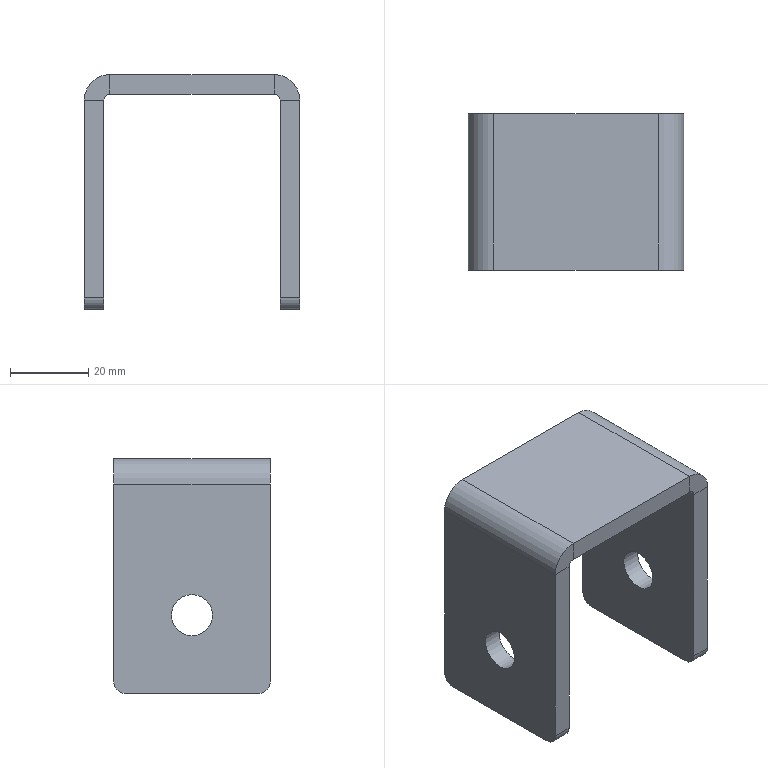Part | STEP file | 6150404 | 1 solid | 28 faces | box 55 x 40 x 60 mm | volume 31409 mm3 | plane 18 | cylinder 10 | commonest cylinder face diameters 6 x4 3 x2 10.5 x2 13 x2
STEP:
#1=CARTESIAN_POINT('',(22.5,3.,-30.));
#2=VERTEX_POINT('',#1);
#3=CARTESIAN_POINT('',(27.5,3.,-30.));
#4=VERTEX_POINT('',#3);
#5=CARTESIAN_POINT('',(-111.1,3.,-30.));
#6=DIRECTION('',(1.,0.,0.));
#7=VECTOR('',#6,1000.);
#8=LINE('',#5,#7);
#9=EDGE_CURVE('',#2,#4,#8,.T.);
#10=ORIENTED_EDGE('',*,*,#9,.T.);
#11=CARTESIAN_POINT('',(27.5,0.,-27.));
#12=VERTEX_POINT('',#11);
#13=CARTESIAN_POINT('',(27.5,3.,-27.));
#14=DIRECTION('',(1.,0.,0.));
#15=DIRECTION('',(0.,0.,1.));
#16=AXIS2_PLACEMENT_3D('',#13,#14,#15);
#17=CIRCLE('',#16,3.);
#18=EDGE_CURVE('',#12,#4,#17,.T.);
#19=ORIENTED_EDGE('',*,*,#18,.F.);
#20=CARTESIAN_POINT('',(22.5,0.,-27.));
#21=VERTEX_POINT('',#20);
#22=CARTESIAN_POINT('',(-111.1,0.,-27.));
#23=DIRECTION('',(1.,0.,0.));
#24=VECTOR('',#23,1000.);
#25=LINE('',#22,#24);
#26=EDGE_CURVE('',#21,#12,#25,.T.);
#27=ORIENTED_EDGE('',*,*,#26,.F.);
#28=CARTESIAN_POINT('',(22.5,3.,-27.));
#29=DIRECTION('',(-1.,0.,0.));
#30=DIRECTION('',(0.,0.,-1.));
#31=AXIS2_PLACEMENT_3D('',#28,#29,#30);
#32=CIRCLE('',#31,3.);
#33=EDGE_CURVE('',#2,#21,#32,.T.);
#34=ORIENTED_EDGE('',*,*,#33,.F.);
#35=EDGE_LOOP('',(#10,#19,#27,#34));
#36=FACE_OUTER_BOUND('',#35,.T.);
#37=CARTESIAN_POINT('',(-111.1,3.,-27.));
#38=DIRECTION('',(1.,0.,0.));
#39=DIRECTION('',(0.,0.,-1.));
#40=AXIS2_PLACEMENT_3D('',#37,#38,#39);
#41=CYLINDRICAL_SURFACE('',#40,3.);
#42=ADVANCED_FACE('',(#36),#41,.T.);
#43=CARTESIAN_POINT('',(22.5,37.,-30.));
#44=VERTEX_POINT('',#43);
#45=CARTESIAN_POINT('',(27.5,37.,-30.));
#46=VERTEX_POINT('',#45);
#47=CARTESIAN_POINT('',(-111.1,37.,-30.));
#48=DIRECTION('',(1.,0.,0.));
#49=VECTOR('',#48,1000.);
#50=LINE('',#47,#49);
#51=EDGE_CURVE('',#44,#46,#50,.T.);
#52=ORIENTED_EDGE('',*,*,#51,.T.);
#53=CARTESIAN_POINT('',(27.5,40.,-30.));
#54=DIRECTION('',(0.,-1.,0.));
#55=VECTOR('',#54,1000.);
#56=LINE('',#53,#55);
#57=EDGE_CURVE('',#46,#4,#56,.T.);
#58=ORIENTED_EDGE('',*,*,#57,.T.);
#59=ORIENTED_EDGE('',*,*,#9,.F.);
#60=CARTESIAN_POINT('',(22.5,40.,-30.));
#61=DIRECTION('',(0.,-1.,0.));
#62=VECTOR('',#61,1000.);
#63=LINE('',#60,#62);
#64=EDGE_CURVE('',#44,#2,#63,.T.);
#65=ORIENTED_EDGE('',*,*,#64,.F.);
#66=EDGE_LOOP('',(#52,#58,#59,#65));
#67=FACE_OUTER_BOUND('',#66,.T.);
#68=CARTESIAN_POINT('',(-111.1,40.,-30.));
#69=DIRECTION('',(0.,0.,1.));
#70=DIRECTION('',(1.,0.,0.));
#71=AXIS2_PLACEMENT_3D('',#68,#69,#70);
#72=PLANE('',#71);
#73=ADVANCED_FACE('',(#67),#72,.F.);
#74=CARTESIAN_POINT('',(22.5,20.,-15.25));
#75=VERTEX_POINT('',#74);
#76=CARTESIAN_POINT('',(22.5,20.,-10.));
#77=DIRECTION('',(1.,0.,0.));
#78=DIRECTION('',(0.,0.,-1.));
#79=AXIS2_PLACEMENT_3D('',#76,#77,#78);
#80=CIRCLE('',#79,5.25);
#81=EDGE_CURVE('',#75,#75,#80,.T.);
#82=ORIENTED_EDGE('',*,*,#81,.F.);
#83=EDGE_LOOP('',(#82));
#84=FACE_OUTER_BOUND('',#83,.T.);
#85=CARTESIAN_POINT('',(27.5,20.,-4.75));
#86=VERTEX_POINT('',#85);
#87=CARTESIAN_POINT('',(27.5,20.,-10.));
#88=DIRECTION('',(-1.,0.,0.));
#89=DIRECTION('',(0.,0.,1.));
#90=AXIS2_PLACEMENT_3D('',#87,#88,#89);
#91=CIRCLE('',#90,5.25);
#92=EDGE_CURVE('',#86,#86,#91,.T.);
#93=ORIENTED_EDGE('',*,*,#92,.F.);
#94=EDGE_LOOP('',(#93));
#95=FACE_OUTER_BOUND('',#94,.T.);
#96=CARTESIAN_POINT('',(36.5,20.,-10.));
#97=DIRECTION('',(-1.,0.,0.));
#98=DIRECTION('',(0.,0.,1.));
#99=AXIS2_PLACEMENT_3D('',#96,#97,#98);
#100=CYLINDRICAL_SURFACE('',#99,5.25);
#101=ADVANCED_FACE('',(#84,#95),#100,.F.);
#102=CARTESIAN_POINT('',(22.5,40.,-27.));
#103=VERTEX_POINT('',#102);
#104=CARTESIAN_POINT('',(27.5,40.,-27.));
#105=VERTEX_POINT('',#104);
#106=CARTESIAN_POINT('',(-111.1,40.,-27.));
#107=DIRECTION('',(1.,0.,0.));
#108=VECTOR('',#107,1000.);
#109=LINE('',#106,#108);
#110=EDGE_CURVE('',#103,#105,#109,.T.);
#111=ORIENTED_EDGE('',*,*,#110,.T.);
#112=CARTESIAN_POINT('',(27.5,37.,-27.));
#113=DIRECTION('',(1.,0.,0.));
#114=DIRECTION('',(0.,0.,1.));
#115=AXIS2_PLACEMENT_3D('',#112,#113,#114);
#116=CIRCLE('',#115,3.);
#117=EDGE_CURVE('',#46,#105,#116,.T.);
#118=ORIENTED_EDGE('',*,*,#117,.F.);
#119=ORIENTED_EDGE('',*,*,#51,.F.);
#120=CARTESIAN_POINT('',(22.5,37.,-27.));
#121=DIRECTION('',(-1.,0.,0.));
#122=DIRECTION('',(0.,0.,-1.));
#123=AXIS2_PLACEMENT_3D('',#120,#121,#122);
#124=CIRCLE('',#123,3.);
#125=EDGE_CURVE('',#103,#44,#124,.T.);
#126=ORIENTED_EDGE('',*,*,#125,.F.);
#127=EDGE_LOOP('',(#111,#118,#119,#126));
#128=FACE_OUTER_BOUND('',#127,.T.);
#129=CARTESIAN_POINT('',(-111.1,37.,-27.));
#130=DIRECTION('',(1.,0.,0.));
#131=DIRECTION('',(0.,0.,-1.));
#132=AXIS2_PLACEMENT_3D('',#129,#130,#131);
#133=CYLINDRICAL_SURFACE('',#132,3.);
#134=ADVANCED_FACE('',(#128),#133,.T.);
#135=CARTESIAN_POINT('',(27.5,40.,23.5));
#136=VERTEX_POINT('',#135);
#137=CARTESIAN_POINT('',(27.5,40.,-30.));
#138=DIRECTION('',(0.,0.,-1.));
#139=VECTOR('',#138,1000.);
#140=LINE('',#137,#139);
#141=EDGE_CURVE('',#136,#105,#140,.T.);
#142=ORIENTED_EDGE('',*,*,#141,.T.);
#143=ORIENTED_EDGE('',*,*,#110,.F.);
#144=CARTESIAN_POINT('',(22.5,40.,23.5));
#145=VERTEX_POINT('',#144);
#146=CARTESIAN_POINT('',(22.5,40.,-30.));
#147=DIRECTION('',(0.,0.,1.));
#148=VECTOR('',#147,1000.);
#149=LINE('',#146,#148);
#150=EDGE_CURVE('',#103,#145,#149,.T.);
#151=ORIENTED_EDGE('',*,*,#150,.T.);
#152=CARTESIAN_POINT('',(-111.1,40.,23.5));
#153=DIRECTION('',(1.,0.,0.));
#154=VECTOR('',#153,1000.);
#155=LINE('',#152,#154);
#156=EDGE_CURVE('',#145,#136,#155,.T.);
#157=ORIENTED_EDGE('',*,*,#156,.T.);
#158=EDGE_LOOP('',(#142,#143,#151,#157));
#159=FACE_OUTER_BOUND('',#158,.T.);
#160=CARTESIAN_POINT('',(-111.1,40.,-30.));
#161=DIRECTION('',(0.,1.,0.));
#162=DIRECTION('',(1.,0.,0.));
#163=AXIS2_PLACEMENT_3D('',#160,#161,#162);
#164=PLANE('',#163);
#165=ADVANCED_FACE('',(#159),#164,.T.);
#166=ORIENTED_EDGE('',*,*,#92,.T.);
#167=EDGE_LOOP('',(#166));
#168=FACE_BOUND('',#167,.T.);
#169=ORIENTED_EDGE('',*,*,#57,.F.);
#170=ORIENTED_EDGE('',*,*,#117,.T.);
#171=ORIENTED_EDGE('',*,*,#141,.F.);
#172=CARTESIAN_POINT('',(27.5,0.,23.5));
#173=VERTEX_POINT('',#172);
#174=CARTESIAN_POINT('',(27.5,40.,23.5));
#175=DIRECTION('',(0.,-1.,0.));
#176=VECTOR('',#175,1000.);
#177=LINE('',#174,#176);
#178=EDGE_CURVE('',#136,#173,#177,.T.);
#179=ORIENTED_EDGE('',*,*,#178,.T.);
#180=CARTESIAN_POINT('',(27.5,0.,-30.));
#181=DIRECTION('',(0.,0.,-1.));
#182=VECTOR('',#181,1000.);
#183=LINE('',#180,#182);
#184=EDGE_CURVE('',#173,#12,#183,.T.);
#185=ORIENTED_EDGE('',*,*,#184,.T.);
#186=ORIENTED_EDGE('',*,*,#18,.T.);
#187=EDGE_LOOP('',(#169,#170,#171,#179,#185,#186));
#188=FACE_OUTER_BOUND('',#187,.T.);
#189=CARTESIAN_POINT('',(27.5,40.,-30.));
#190=DIRECTION('',(-1.,0.,0.));
#191=DIRECTION('',(0.,0.,1.));
#192=AXIS2_PLACEMENT_3D('',#189,#190,#191);
#193=PLANE('',#192);
#194=ADVANCED_FACE('',(#168,#188),#193,.F.);
#195=ORIENTED_EDGE('',*,*,#26,.T.);
#196=ORIENTED_EDGE('',*,*,#184,.F.);
#197=CARTESIAN_POINT('',(22.5,0.,23.5));
#198=VERTEX_POINT('',#197);
#199=CARTESIAN_POINT('',(-111.1,0.,23.5));
#200=DIRECTION('',(1.,0.,0.));
#201=VECTOR('',#200,1000.);
#202=LINE('',#199,#201);
#203=EDGE_CURVE('',#198,#173,#202,.T.);
#204=ORIENTED_EDGE('',*,*,#203,.F.);
#205=CARTESIAN_POINT('',(22.5,0.,-30.));
#206=DIRECTION('',(0.,0.,1.));
#207=VECTOR('',#206,1000.);
#208=LINE('',#205,#207);
#209=EDGE_CURVE('',#21,#198,#208,.T.);
#210=ORIENTED_EDGE('',*,*,#209,.F.);
#211=EDGE_LOOP('',(#195,#196,#204,#210));
#212=FACE_OUTER_BOUND('',#211,.T.);
#213=CARTESIAN_POINT('',(-111.1,0.,-30.));
#214=DIRECTION('',(0.,1.,0.));
#215=DIRECTION('',(1.,0.,0.));
#216=AXIS2_PLACEMENT_3D('',#213,#214,#215);
#217=PLANE('',#216);
#218=ADVANCED_FACE('',(#212),#217,.F.);
#219=ORIENTED_EDGE('',*,*,#81,.T.);
#220=EDGE_LOOP('',(#219));
#221=FACE_BOUND('',#220,.T.);
#222=ORIENTED_EDGE('',*,*,#150,.F.);
#223=ORIENTED_EDGE('',*,*,#125,.T.);
#224=ORIENTED_EDGE('',*,*,#64,.T.);
#225=ORIENTED_EDGE('',*,*,#33,.T.);
#226=ORIENTED_EDGE('',*,*,#209,.T.);
#227=CARTESIAN_POINT('',(22.5,40.,23.5));
#228=DIRECTION('',(0.,-1.,0.));
#229=VECTOR('',#228,1000.);
#230=LINE('',#227,#229);
#231=EDGE_CURVE('',#145,#198,#230,.T.);
#232=ORIENTED_EDGE('',*,*,#231,.F.);
#233=EDGE_LOOP('',(#222,#223,#224,#225,#226,#232));
#234=FACE_OUTER_BOUND('',#233,.T.);
#235=CARTESIAN_POINT('',(22.5,40.,-30.));
#236=DIRECTION('',(1.,0.,0.));
#237=DIRECTION('',(0.,0.,-1.));
#238=AXIS2_PLACEMENT_3D('',#235,#236,#237);
#239=PLANE('',#238);
#240=ADVANCED_FACE('',(#221,#234),#239,.F.);
#241=CARTESIAN_POINT('',(-22.5,37.,-30.));
#242=VERTEX_POINT('',#241);
#243=CARTESIAN_POINT('',(-27.5,37.,-30.));
#244=VERTEX_POINT('',#243);
#245=CARTESIAN_POINT('',(111.1,37.,-30.));
#246=DIRECTION('',(-1.,0.,0.));
#247=VECTOR('',#246,1000.);
#248=LINE('',#245,#247);
#249=EDGE_CURVE('',#242,#244,#248,.T.);
#250=ORIENTED_EDGE('',*,*,#249,.T.);
#251=CARTESIAN_POINT('',(-27.5,40.,-27.));
#252=VERTEX_POINT('',#251);
#253=CARTESIAN_POINT('',(-27.5,37.,-27.));
#254=DIRECTION('',(-1.,0.,0.));
#255=DIRECTION('',(0.,0.,-1.));
#256=AXIS2_PLACEMENT_3D('',#253,#254,#255);
#257=CIRCLE('',#256,3.);
#258=EDGE_CURVE('',#252,#244,#257,.T.);
#259=ORIENTED_EDGE('',*,*,#258,.F.);
#260=CARTESIAN_POINT('',(-22.5,40.,-27.));
#261=VERTEX_POINT('',#260);
#262=CARTESIAN_POINT('',(111.1,40.,-27.));
#263=DIRECTION('',(-1.,0.,0.));
#264=VECTOR('',#263,1000.);
#265=LINE('',#262,#264);
#266=EDGE_CURVE('',#261,#252,#265,.T.);
#267=ORIENTED_EDGE('',*,*,#266,.F.);
#268=CARTESIAN_POINT('',(-22.5,37.,-27.));
#269=DIRECTION('',(1.,0.,0.));
#270=DIRECTION('',(0.,0.,1.));
#271=AXIS2_PLACEMENT_3D('',#268,#269,#270);
#272=CIRCLE('',#271,3.);
#273=EDGE_CURVE('',#242,#261,#272,.T.);
#274=ORIENTED_EDGE('',*,*,#273,.F.);
#275=EDGE_LOOP('',(#250,#259,#267,#274));
#276=FACE_OUTER_BOUND('',#275,.T.);
#277=CARTESIAN_POINT('',(111.1,37.,-27.));
#278=DIRECTION('',(-1.,0.,0.));
#279=DIRECTION('',(0.,0.,1.));
#280=AXIS2_PLACEMENT_3D('',#277,#278,#279);
#281=CYLINDRICAL_SURFACE('',#280,3.);
#282=ADVANCED_FACE('',(#276),#281,.T.);
#283=CARTESIAN_POINT('',(-27.5,3.,-30.));
#284=VERTEX_POINT('',#283);
#285=CARTESIAN_POINT('',(-27.5,40.,-30.));
#286=DIRECTION('',(0.,-1.,0.));
#287=VECTOR('',#286,1000.);
#288=LINE('',#285,#287);
#289=EDGE_CURVE('',#244,#284,#288,.T.);
#290=ORIENTED_EDGE('',*,*,#289,.F.);
#291=ORIENTED_EDGE('',*,*,#249,.F.);
#292=CARTESIAN_POINT('',(-22.5,3.,-30.));
#293=VERTEX_POINT('',#292);
#294=CARTESIAN_POINT('',(-22.5,40.,-30.));
#295=DIRECTION('',(0.,-1.,0.));
#296=VECTOR('',#295,1000.);
#297=LINE('',#294,#296);
#298=EDGE_CURVE('',#242,#293,#297,.T.);
#299=ORIENTED_EDGE('',*,*,#298,.T.);
#300=CARTESIAN_POINT('',(111.1,3.,-30.));
#301=DIRECTION('',(-1.,0.,0.));
#302=VECTOR('',#301,1000.);
#303=LINE('',#300,#302);
#304=EDGE_CURVE('',#293,#284,#303,.T.);
#305=ORIENTED_EDGE('',*,*,#304,.T.);
#306=EDGE_LOOP('',(#290,#291,#299,#305));
#307=FACE_OUTER_BOUND('',#306,.T.);
#308=CARTESIAN_POINT('',(111.1,40.,-30.));
#309=DIRECTION('',(0.,0.,-1.));
#310=DIRECTION('',(-1.,0.,0.));
#311=AXIS2_PLACEMENT_3D('',#308,#309,#310);
#312=PLANE('',#311);
#313=ADVANCED_FACE('',(#307),#312,.T.);
#314=CARTESIAN_POINT('',(-27.5,20.,-4.75));
#315=VERTEX_POINT('',#314);
#316=CARTESIAN_POINT('',(-27.5,20.,-10.));
#317=DIRECTION('',(-1.,0.,0.));
#318=DIRECTION('',(0.,0.,1.));
#319=AXIS2_PLACEMENT_3D('',#316,#317,#318);
#320=CIRCLE('',#319,5.25);
#321=EDGE_CURVE('',#315,#315,#320,.T.);
#322=ORIENTED_EDGE('',*,*,#321,.T.);
#323=EDGE_LOOP('',(#322));
#324=FACE_OUTER_BOUND('',#323,.T.);
#325=CARTESIAN_POINT('',(-22.5,20.,-4.75));
#326=VERTEX_POINT('',#325);
#327=CARTESIAN_POINT('',(-22.5,20.,-10.));
#328=DIRECTION('',(-1.,0.,0.));
#329=DIRECTION('',(0.,0.,1.));
#330=AXIS2_PLACEMENT_3D('',#327,#328,#329);
#331=CIRCLE('',#330,5.25);
#332=EDGE_CURVE('',#326,#326,#331,.T.);
#333=ORIENTED_EDGE('',*,*,#332,.F.);
#334=EDGE_LOOP('',(#333));
#335=FACE_OUTER_BOUND('',#334,.T.);
#336=CARTESIAN_POINT('',(36.5,20.,-10.));
#337=DIRECTION('',(-1.,0.,0.));
#338=DIRECTION('',(0.,0.,1.));
#339=AXIS2_PLACEMENT_3D('',#336,#337,#338);
#340=CYLINDRICAL_SURFACE('',#339,5.25);
#341=ADVANCED_FACE('',(#324,#335),#340,.F.);
#342=CARTESIAN_POINT('',(-22.5,0.,-27.));
#343=VERTEX_POINT('',#342);
#344=CARTESIAN_POINT('',(-27.5,0.,-27.));
#345=VERTEX_POINT('',#344);
#346=CARTESIAN_POINT('',(111.1,0.,-27.));
#347=DIRECTION('',(-1.,0.,0.));
#348=VECTOR('',#347,1000.);
#349=LINE('',#346,#348);
#350=EDGE_CURVE('',#343,#345,#349,.T.);
#351=ORIENTED_EDGE('',*,*,#350,.T.);
#352=CARTESIAN_POINT('',(-27.5,3.,-27.));
#353=DIRECTION('',(-1.,0.,0.));
#354=DIRECTION('',(0.,0.,-1.));
#355=AXIS2_PLACEMENT_3D('',#352,#353,#354);
#356=CIRCLE('',#355,3.);
#357=EDGE_CURVE('',#284,#345,#356,.T.);
#358=ORIENTED_EDGE('',*,*,#357,.F.);
#359=ORIENTED_EDGE('',*,*,#304,.F.);
#360=CARTESIAN_POINT('',(-22.5,3.,-27.));
#361=DIRECTION('',(1.,0.,0.));
#362=DIRECTION('',(0.,0.,1.));
#363=AXIS2_PLACEMENT_3D('',#360,#361,#362);
#364=CIRCLE('',#363,3.);
#365=EDGE_CURVE('',#343,#293,#364,.T.);
#366=ORIENTED_EDGE('',*,*,#365,.F.);
#367=EDGE_LOOP('',(#351,#358,#359,#366));
#368=FACE_OUTER_BOUND('',#367,.T.);
#369=CARTESIAN_POINT('',(111.1,3.,-27.));
#370=DIRECTION('',(-1.,0.,0.));
#371=DIRECTION('',(0.,0.,1.));
#372=AXIS2_PLACEMENT_3D('',#369,#370,#371);
#373=CYLINDRICAL_SURFACE('',#372,3.);
#374=ADVANCED_FACE('',(#368),#373,.T.);
#375=CARTESIAN_POINT('',(-22.5,0.,23.5));
#376=VERTEX_POINT('',#375);
#377=CARTESIAN_POINT('',(-27.5,0.,23.5));
#378=VERTEX_POINT('',#377);
#379=CARTESIAN_POINT('',(111.1,0.,23.5));
#380=DIRECTION('',(-1.,0.,0.));
#381=VECTOR('',#380,1000.);
#382=LINE('',#379,#381);
#383=EDGE_CURVE('',#376,#378,#382,.T.);
#384=ORIENTED_EDGE('',*,*,#383,.T.);
#385=CARTESIAN_POINT('',(-27.5,0.,-30.));
#386=DIRECTION('',(0.,0.,1.));
#387=VECTOR('',#386,1000.);
#388=LINE('',#385,#387);
#389=EDGE_CURVE('',#345,#378,#388,.T.);
#390=ORIENTED_EDGE('',*,*,#389,.F.);
#391=ORIENTED_EDGE('',*,*,#350,.F.);
#392=CARTESIAN_POINT('',(-22.5,0.,-30.));
#393=DIRECTION('',(0.,0.,-1.));
#394=VECTOR('',#393,1000.);
#395=LINE('',#392,#394);
#396=EDGE_CURVE('',#376,#343,#395,.T.);
#397=ORIENTED_EDGE('',*,*,#396,.F.);
#398=EDGE_LOOP('',(#384,#390,#391,#397));
#399=FACE_OUTER_BOUND('',#398,.T.);
#400=CARTESIAN_POINT('',(111.1,0.,-30.));
#401=DIRECTION('',(0.,1.,0.));
#402=DIRECTION('',(-1.,0.,0.));
#403=AXIS2_PLACEMENT_3D('',#400,#401,#402);
#404=PLANE('',#403);
#405=ADVANCED_FACE('',(#399),#404,.F.);
#406=ORIENTED_EDGE('',*,*,#321,.F.);
#407=EDGE_LOOP('',(#406));
#408=FACE_BOUND('',#407,.T.);
#409=ORIENTED_EDGE('',*,*,#289,.T.);
#410=ORIENTED_EDGE('',*,*,#357,.T.);
#411=ORIENTED_EDGE('',*,*,#389,.T.);
#412=CARTESIAN_POINT('',(-27.5,40.,23.5));
#413=VERTEX_POINT('',#412);
#414=CARTESIAN_POINT('',(-27.5,40.,23.5));
#415=DIRECTION('',(0.,-1.,0.));
#416=VECTOR('',#415,1000.);
#417=LINE('',#414,#416);
#418=EDGE_CURVE('',#413,#378,#417,.T.);
#419=ORIENTED_EDGE('',*,*,#418,.F.);
#420=CARTESIAN_POINT('',(-27.5,40.,-30.));
#421=DIRECTION('',(0.,0.,1.));
#422=VECTOR('',#421,1000.);
#423=LINE('',#420,#422);
#424=EDGE_CURVE('',#252,#413,#423,.T.);
#425=ORIENTED_EDGE('',*,*,#424,.F.);
#426=ORIENTED_EDGE('',*,*,#258,.T.);
#427=EDGE_LOOP('',(#409,#410,#411,#419,#425,#426));
#428=FACE_OUTER_BOUND('',#427,.T.);
#429=CARTESIAN_POINT('',(-27.5,40.,-30.));
#430=DIRECTION('',(1.,0.,0.));
#431=DIRECTION('',(0.,0.,-1.));
#432=AXIS2_PLACEMENT_3D('',#429,#430,#431);
#433=PLANE('',#432);
#434=ADVANCED_FACE('',(#408,#428),#433,.F.);
#435=ORIENTED_EDGE('',*,*,#424,.T.);
#436=CARTESIAN_POINT('',(-22.5,40.,23.5));
#437=VERTEX_POINT('',#436);
#438=CARTESIAN_POINT('',(111.1,40.,23.5));
#439=DIRECTION('',(-1.,0.,0.));
#440=VECTOR('',#439,1000.);
#441=LINE('',#438,#440);
#442=EDGE_CURVE('',#437,#413,#441,.T.);
#443=ORIENTED_EDGE('',*,*,#442,.F.);
#444=CARTESIAN_POINT('',(-22.5,40.,-30.));
#445=DIRECTION('',(0.,0.,-1.));
#446=VECTOR('',#445,1000.);
#447=LINE('',#444,#446);
#448=EDGE_CURVE('',#437,#261,#447,.T.);
#449=ORIENTED_EDGE('',*,*,#448,.T.);
#450=ORIENTED_EDGE('',*,*,#266,.T.);
#451=EDGE_LOOP('',(#435,#443,#449,#450));
#452=FACE_OUTER_BOUND('',#451,.T.);
#453=CARTESIAN_POINT('',(111.1,40.,-30.));
#454=DIRECTION('',(0.,1.,0.));
#455=DIRECTION('',(-1.,0.,0.));
#456=AXIS2_PLACEMENT_3D('',#453,#454,#455);
#457=PLANE('',#456);
#458=ADVANCED_FACE('',(#452),#457,.T.);
#459=ORIENTED_EDGE('',*,*,#332,.T.);
#460=EDGE_LOOP('',(#459));
#461=FACE_BOUND('',#460,.T.);
#462=ORIENTED_EDGE('',*,*,#396,.T.);
#463=ORIENTED_EDGE('',*,*,#365,.T.);
#464=ORIENTED_EDGE('',*,*,#298,.F.);
#465=ORIENTED_EDGE('',*,*,#273,.T.);
#466=ORIENTED_EDGE('',*,*,#448,.F.);
#467=CARTESIAN_POINT('',(-22.5,40.,23.5));
#468=DIRECTION('',(0.,-1.,0.));
#469=VECTOR('',#468,1000.);
#470=LINE('',#467,#469);
#471=EDGE_CURVE('',#437,#376,#470,.T.);
#472=ORIENTED_EDGE('',*,*,#471,.T.);
#473=EDGE_LOOP('',(#462,#463,#464,#465,#466,#472));
#474=FACE_OUTER_BOUND('',#473,.T.);
#475=CARTESIAN_POINT('',(-22.5,40.,-30.));
#476=DIRECTION('',(-1.,0.,0.));
#477=DIRECTION('',(0.,0.,1.));
#478=AXIS2_PLACEMENT_3D('',#475,#476,#477);
#479=PLANE('',#478);
#480=ADVANCED_FACE('',(#461,#474),#479,.F.);
#481=CARTESIAN_POINT('',(-21.,0.,30.));
#482=VERTEX_POINT('',#481);
#483=CARTESIAN_POINT('',(21.,0.,30.));
#484=VERTEX_POINT('',#483);
#485=CARTESIAN_POINT('',(-21.,0.,30.));
#486=DIRECTION('',(1.,0.,0.));
#487=VECTOR('',#486,1000.);
#488=LINE('',#485,#487);
#489=EDGE_CURVE('',#482,#484,#488,.T.);
#490=ORIENTED_EDGE('',*,*,#489,.T.);
#491=CARTESIAN_POINT('',(21.,40.,30.));
#492=VERTEX_POINT('',#491);
#493=CARTESIAN_POINT('',(21.,40.,30.));
#494=DIRECTION('',(0.,-1.,0.));
#495=VECTOR('',#494,1000.);
#496=LINE('',#493,#495);
#497=EDGE_CURVE('',#492,#484,#496,.T.);
#498=ORIENTED_EDGE('',*,*,#497,.F.);
#499=CARTESIAN_POINT('',(-21.,40.,30.));
#500=VERTEX_POINT('',#499);
#501=CARTESIAN_POINT('',(-21.,40.,30.));
#502=DIRECTION('',(1.,0.,0.));
#503=VECTOR('',#502,1000.);
#504=LINE('',#501,#503);
#505=EDGE_CURVE('',#500,#492,#504,.T.);
#506=ORIENTED_EDGE('',*,*,#505,.F.);
#507=CARTESIAN_POINT('',(-21.,40.,30.));
#508=DIRECTION('',(0.,-1.,0.));
#509=VECTOR('',#508,1000.);
#510=LINE('',#507,#509);
#511=EDGE_CURVE('',#500,#482,#510,.T.);
#512=ORIENTED_EDGE('',*,*,#511,.T.);
#513=EDGE_LOOP('',(#490,#498,#506,#512));
#514=FACE_OUTER_BOUND('',#513,.T.);
#515=CARTESIAN_POINT('',(-21.,40.,30.));
#516=DIRECTION('',(0.,0.,-1.));
#517=DIRECTION('',(-1.,0.,0.));
#518=AXIS2_PLACEMENT_3D('',#515,#516,#517);
#519=PLANE('',#518);
#520=ADVANCED_FACE('',(#514),#519,.F.);
#521=CARTESIAN_POINT('',(21.,0.,25.));
#522=VERTEX_POINT('',#521);
#523=CARTESIAN_POINT('',(-21.,0.,25.));
#524=VERTEX_POINT('',#523);
#525=CARTESIAN_POINT('',(-21.,0.,25.));
#526=DIRECTION('',(-1.,0.,0.));
#527=VECTOR('',#526,1000.);
#528=LINE('',#525,#527);
#529=EDGE_CURVE('',#522,#524,#528,.T.);
#530=ORIENTED_EDGE('',*,*,#529,.T.);
#531=CARTESIAN_POINT('',(-21.,40.,25.));
#532=VERTEX_POINT('',#531);
#533=CARTESIAN_POINT('',(-21.,40.,25.));
#534=DIRECTION('',(0.,-1.,0.));
#535=VECTOR('',#534,1000.);
#536=LINE('',#533,#535);
#537=EDGE_CURVE('',#532,#524,#536,.T.);
#538=ORIENTED_EDGE('',*,*,#537,.F.);
#539=CARTESIAN_POINT('',(21.,40.,25.));
#540=VERTEX_POINT('',#539);
#541=CARTESIAN_POINT('',(-21.,40.,25.));
#542=DIRECTION('',(-1.,0.,0.));
#543=VECTOR('',#542,1000.);
#544=LINE('',#541,#543);
#545=EDGE_CURVE('',#540,#532,#544,.T.);
#546=ORIENTED_EDGE('',*,*,#545,.F.);
#547=CARTESIAN_POINT('',(21.,40.,25.));
#548=DIRECTION('',(0.,-1.,0.));
#549=VECTOR('',#548,1000.);
#550=LINE('',#547,#549);
#551=EDGE_CURVE('',#540,#522,#550,.T.);
#552=ORIENTED_EDGE('',*,*,#551,.T.);
#553=EDGE_LOOP('',(#530,#538,#546,#552));
#554=FACE_OUTER_BOUND('',#553,.T.);
#555=CARTESIAN_POINT('',(-21.,40.,25.));
#556=DIRECTION('',(0.,0.,1.));
#557=DIRECTION('',(1.,0.,0.));
#558=AXIS2_PLACEMENT_3D('',#555,#556,#557);
#559=PLANE('',#558);
#560=ADVANCED_FACE('',(#554),#559,.F.);
#561=CARTESIAN_POINT('',(21.,0.,-91.));
#562=DIRECTION('',(0.,0.,1.));
#563=VECTOR('',#562,1000.);
#564=LINE('',#561,#563);
#565=EDGE_CURVE('',#522,#484,#564,.T.);
#566=ORIENTED_EDGE('',*,*,#565,.T.);
#567=ORIENTED_EDGE('',*,*,#489,.F.);
#568=CARTESIAN_POINT('',(-21.,0.,-91.));
#569=DIRECTION('',(0.,0.,1.));
#570=VECTOR('',#569,1000.);
#571=LINE('',#568,#570);
#572=EDGE_CURVE('',#524,#482,#571,.T.);
#573=ORIENTED_EDGE('',*,*,#572,.F.);
#574=ORIENTED_EDGE('',*,*,#529,.F.);
#575=EDGE_LOOP('',(#566,#567,#573,#574));
#576=FACE_OUTER_BOUND('',#575,.T.);
#577=CARTESIAN_POINT('',(-21.,0.,-91.));
#578=DIRECTION('',(0.,1.,0.));
#579=DIRECTION('',(0.,0.,1.));
#580=AXIS2_PLACEMENT_3D('',#577,#578,#579);
#581=PLANE('',#580);
#582=ADVANCED_FACE('',(#576),#581,.F.);
#583=ORIENTED_EDGE('',*,*,#505,.T.);
#584=CARTESIAN_POINT('',(21.,40.,-91.));
#585=DIRECTION('',(0.,0.,1.));
#586=VECTOR('',#585,1000.);
#587=LINE('',#584,#586);
#588=EDGE_CURVE('',#540,#492,#587,.T.);
#589=ORIENTED_EDGE('',*,*,#588,.F.);
#590=ORIENTED_EDGE('',*,*,#545,.T.);
#591=CARTESIAN_POINT('',(-21.,40.,-91.));
#592=DIRECTION('',(0.,0.,1.));
#593=VECTOR('',#592,1000.);
#594=LINE('',#591,#593);
#595=EDGE_CURVE('',#532,#500,#594,.T.);
#596=ORIENTED_EDGE('',*,*,#595,.T.);
#597=EDGE_LOOP('',(#583,#589,#590,#596));
#598=FACE_OUTER_BOUND('',#597,.T.);
#599=CARTESIAN_POINT('',(-21.,40.,-91.));
#600=DIRECTION('',(0.,1.,0.));
#601=DIRECTION('',(0.,0.,1.));
#602=AXIS2_PLACEMENT_3D('',#599,#600,#601);
#603=PLANE('',#602);
#604=ADVANCED_FACE('',(#598),#603,.T.);
#605=ORIENTED_EDGE('',*,*,#383,.F.);
#606=CARTESIAN_POINT('',(-21.,0.,23.5));
#607=DIRECTION('',(0.,1.,0.));
#608=DIRECTION('',(0.,0.,1.));
#609=AXIS2_PLACEMENT_3D('',#606,#607,#608);
#610=CIRCLE('',#609,1.5);
#611=EDGE_CURVE('',#376,#524,#610,.T.);
#612=ORIENTED_EDGE('',*,*,#611,.T.);
#613=ORIENTED_EDGE('',*,*,#572,.T.);
#614=CARTESIAN_POINT('',(-21.,0.,23.5));
#615=DIRECTION('',(0.,1.,0.));
#616=DIRECTION('',(0.,0.,1.));
#617=AXIS2_PLACEMENT_3D('',#614,#615,#616);
#618=CIRCLE('',#617,6.5);
#619=EDGE_CURVE('',#378,#482,#618,.T.);
#620=ORIENTED_EDGE('',*,*,#619,.F.);
#621=EDGE_LOOP('',(#605,#612,#613,#620));
#622=FACE_OUTER_BOUND('',#621,.T.);
#623=CARTESIAN_POINT('',(-21.,0.,23.5));
#624=DIRECTION('',(0.,-1.,0.));
#625=DIRECTION('',(0.,0.,-1.));
#626=AXIS2_PLACEMENT_3D('',#623,#624,#625);
#627=PLANE('',#626);
#628=ADVANCED_FACE('',(#622),#627,.T.);
#629=CARTESIAN_POINT('',(-21.,40.,23.5));
#630=DIRECTION('',(0.,-1.,0.));
#631=DIRECTION('',(0.,0.,1.));
#632=AXIS2_PLACEMENT_3D('',#629,#630,#631);
#633=CIRCLE('',#632,1.5);
#634=EDGE_CURVE('',#532,#437,#633,.T.);
#635=ORIENTED_EDGE('',*,*,#634,.T.);
#636=ORIENTED_EDGE('',*,*,#442,.T.);
#637=CARTESIAN_POINT('',(-21.,40.,23.5));
#638=DIRECTION('',(0.,-1.,0.));
#639=DIRECTION('',(0.,0.,1.));
#640=AXIS2_PLACEMENT_3D('',#637,#638,#639);
#641=CIRCLE('',#640,6.5);
#642=EDGE_CURVE('',#500,#413,#641,.T.);
#643=ORIENTED_EDGE('',*,*,#642,.F.);
#644=ORIENTED_EDGE('',*,*,#595,.F.);
#645=EDGE_LOOP('',(#635,#636,#643,#644));
#646=FACE_OUTER_BOUND('',#645,.T.);
#647=CARTESIAN_POINT('',(-21.,40.,23.5));
#648=DIRECTION('',(0.,1.,0.));
#649=DIRECTION('',(0.,0.,1.));
#650=AXIS2_PLACEMENT_3D('',#647,#648,#649);
#651=PLANE('',#650);
#652=ADVANCED_FACE('',(#646),#651,.T.);
#653=ORIENTED_EDGE('',*,*,#511,.F.);
#654=ORIENTED_EDGE('',*,*,#642,.T.);
#655=ORIENTED_EDGE('',*,*,#418,.T.);
#656=ORIENTED_EDGE('',*,*,#619,.T.);
#657=EDGE_LOOP('',(#653,#654,#655,#656));
#658=FACE_OUTER_BOUND('',#657,.T.);
#659=CARTESIAN_POINT('',(-21.,-166.519,23.5));
#660=DIRECTION('',(0.,1.,0.));
#661=DIRECTION('',(0.,0.,1.));
#662=AXIS2_PLACEMENT_3D('',#659,#660,#661);
#663=CYLINDRICAL_SURFACE('',#662,6.5);
#664=ADVANCED_FACE('',(#658),#663,.T.);
#665=ORIENTED_EDGE('',*,*,#537,.T.);
#666=ORIENTED_EDGE('',*,*,#611,.F.);
#667=ORIENTED_EDGE('',*,*,#471,.F.);
#668=ORIENTED_EDGE('',*,*,#634,.F.);
#669=EDGE_LOOP('',(#665,#666,#667,#668));
#670=FACE_OUTER_BOUND('',#669,.T.);
#671=CARTESIAN_POINT('',(-21.,-166.519,23.5));
#672=DIRECTION('',(0.,1.,0.));
#673=DIRECTION('',(0.,0.,1.));
#674=AXIS2_PLACEMENT_3D('',#671,#672,#673);
#675=CYLINDRICAL_SURFACE('',#674,1.5);
#676=ADVANCED_FACE('',(#670),#675,.F.);
#677=ORIENTED_EDGE('',*,*,#565,.F.);
#678=CARTESIAN_POINT('',(21.,0.,23.5));
#679=DIRECTION('',(0.,1.,0.));
#680=DIRECTION('',(0.,0.,-1.));
#681=AXIS2_PLACEMENT_3D('',#678,#679,#680);
#682=CIRCLE('',#681,1.5);
#683=EDGE_CURVE('',#522,#198,#682,.T.);
#684=ORIENTED_EDGE('',*,*,#683,.T.);
#685=ORIENTED_EDGE('',*,*,#203,.T.);
#686=CARTESIAN_POINT('',(21.,0.,23.5));
#687=DIRECTION('',(0.,1.,0.));
#688=DIRECTION('',(0.,0.,-1.));
#689=AXIS2_PLACEMENT_3D('',#686,#687,#688);
#690=CIRCLE('',#689,6.5);
#691=EDGE_CURVE('',#484,#173,#690,.T.);
#692=ORIENTED_EDGE('',*,*,#691,.F.);
#693=EDGE_LOOP('',(#677,#684,#685,#692));
#694=FACE_OUTER_BOUND('',#693,.T.);
#695=CARTESIAN_POINT('',(21.,0.,23.5));
#696=DIRECTION('',(0.,-1.,0.));
#697=DIRECTION('',(0.,0.,-1.));
#698=AXIS2_PLACEMENT_3D('',#695,#696,#697);
#699=PLANE('',#698);
#700=ADVANCED_FACE('',(#694),#699,.T.);
#701=ORIENTED_EDGE('',*,*,#156,.F.);
#702=CARTESIAN_POINT('',(21.,40.,23.5));
#703=DIRECTION('',(0.,-1.,0.));
#704=DIRECTION('',(0.,0.,-1.));
#705=AXIS2_PLACEMENT_3D('',#702,#703,#704);
#706=CIRCLE('',#705,1.5);
#707=EDGE_CURVE('',#145,#540,#706,.T.);
#708=ORIENTED_EDGE('',*,*,#707,.T.);
#709=ORIENTED_EDGE('',*,*,#588,.T.);
#710=CARTESIAN_POINT('',(21.,40.,23.5));
#711=DIRECTION('',(0.,-1.,0.));
#712=DIRECTION('',(0.,0.,-1.));
#713=AXIS2_PLACEMENT_3D('',#710,#711,#712);
#714=CIRCLE('',#713,6.5);
#715=EDGE_CURVE('',#136,#492,#714,.T.);
#716=ORIENTED_EDGE('',*,*,#715,.F.);
#717=EDGE_LOOP('',(#701,#708,#709,#716));
#718=FACE_OUTER_BOUND('',#717,.T.);
#719=CARTESIAN_POINT('',(21.,40.,23.5));
#720=DIRECTION('',(0.,1.,0.));
#721=DIRECTION('',(0.,0.,1.));
#722=AXIS2_PLACEMENT_3D('',#719,#720,#721);
#723=PLANE('',#722);
#724=ADVANCED_FACE('',(#718),#723,.T.);
#725=ORIENTED_EDGE('',*,*,#715,.T.);
#726=ORIENTED_EDGE('',*,*,#497,.T.);
#727=ORIENTED_EDGE('',*,*,#691,.T.);
#728=ORIENTED_EDGE('',*,*,#178,.F.);
#729=EDGE_LOOP('',(#725,#726,#727,#728));
#730=FACE_OUTER_BOUND('',#729,.T.);
#731=CARTESIAN_POINT('',(21.,170.097,23.5));
#732=DIRECTION('',(0.,-1.,0.));
#733=DIRECTION('',(0.,0.,-1.));
#734=AXIS2_PLACEMENT_3D('',#731,#732,#733);
#735=CYLINDRICAL_SURFACE('',#734,6.5);
#736=ADVANCED_FACE('',(#730),#735,.T.);
#737=ORIENTED_EDGE('',*,*,#707,.F.);
#738=ORIENTED_EDGE('',*,*,#231,.T.);
#739=ORIENTED_EDGE('',*,*,#683,.F.);
#740=ORIENTED_EDGE('',*,*,#551,.F.);
#741=EDGE_LOOP('',(#737,#738,#739,#740));
#742=FACE_OUTER_BOUND('',#741,.T.);
#743=CARTESIAN_POINT('',(21.,170.097,23.5));
#744=DIRECTION('',(0.,-1.,0.));
#745=DIRECTION('',(0.,0.,-1.));
#746=AXIS2_PLACEMENT_3D('',#743,#744,#745);
#747=CYLINDRICAL_SURFACE('',#746,1.5);
#748=ADVANCED_FACE('',(#742),#747,.F.);
#749=CLOSED_SHELL('',(#42,#73,#101,#134,#165,#194,#218,#240,#282,#313,#341,#374,#405,#434,#458,#480,#520,#560,#582,#604,#628,#652,#664,#676,#700,#724,#736,#748));
#750=MANIFOLD_SOLID_BREP('',#749);
#751=CARTESIAN_POINT('',(0.,0.,0.));
#752=DIRECTION('',(0.,0.,1.));
#753=DIRECTION('',(1.,0.,0.));
#754=AXIS2_PLACEMENT_3D('',#751,#752,#753);
#755=(LENGTH_UNIT()NAMED_UNIT(*)SI_UNIT(.MILLI.,.METRE.));
#756=UNCERTAINTY_MEASURE_WITH_UNIT(LENGTH_MEASURE(0.00001),#755,'','');
#757=(NAMED_UNIT(*)PLANE_ANGLE_UNIT()SI_UNIT($,.RADIAN.));
#758=(NAMED_UNIT(*)SI_UNIT($,.STERADIAN.)SOLID_ANGLE_UNIT());
#759=(GEOMETRIC_REPRESENTATION_CONTEXT(3)GLOBAL_UNCERTAINTY_ASSIGNED_CONTEXT((#756))GLOBAL_UNIT_ASSIGNED_CONTEXT((#755,#757,#758))REPRESENTATION_CONTEXT('',''));
#760=ADVANCED_BREP_SHAPE_REPRESENTATION('',(#750,#754),#759);